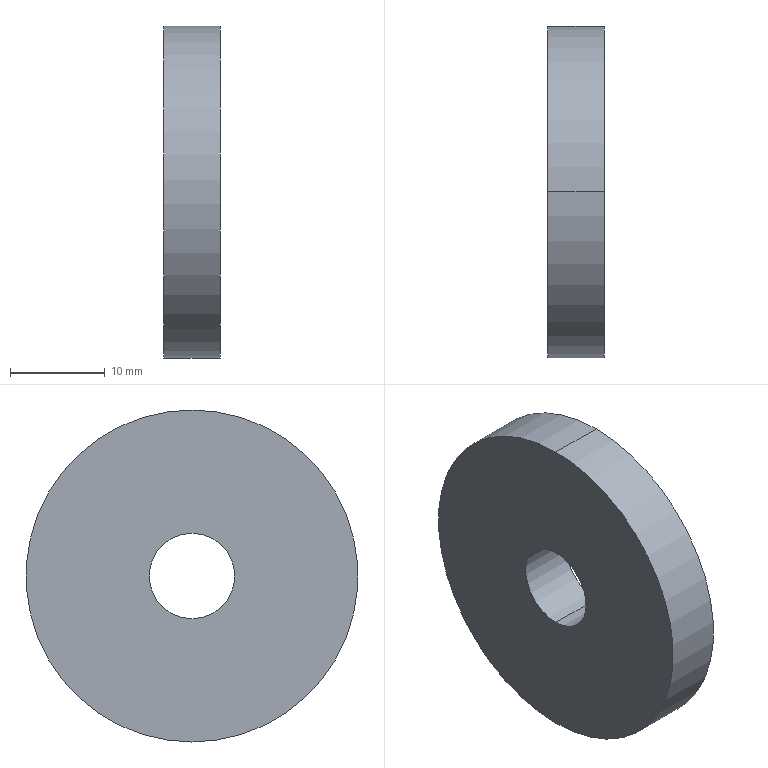Part | SolidWorks | features Extrusion 1 | 1 solid | 6 faces | box 6 x 35 x 35 mm | volume 5391 mm3 | cylinder 4 | plane 2 | commonest cylinder face diameters 9 x2 35 x2
STEP:
#1=CARTESIAN_POINT('',(6.,0.,4.5));
#2=VERTEX_POINT('',#1);
#3=CARTESIAN_POINT('',(6.,0.,-4.5));
#4=VERTEX_POINT('',#3);
#5=CARTESIAN_POINT('',(6.,0.,0.));
#6=DIRECTION('',(1.,0.,0.));
#7=DIRECTION('',(0.,0.,-1.));
#8=AXIS2_PLACEMENT_3D('',#5,#6,#7);
#9=CIRCLE('',#8,4.5);
#10=EDGE_CURVE('',#2,#4,#9,.T.);
#11=ORIENTED_EDGE('',*,*,#10,.T.);
#12=CARTESIAN_POINT('',(0.,0.,-4.5));
#13=VERTEX_POINT('',#12);
#14=CARTESIAN_POINT('',(6.,0.,-4.5));
#15=DIRECTION('',(-1.,0.,0.));
#16=VECTOR('',#15,1000.);
#17=LINE('',#14,#16);
#18=EDGE_CURVE('',#4,#13,#17,.T.);
#19=ORIENTED_EDGE('',*,*,#18,.T.);
#20=CARTESIAN_POINT('',(0.,0.,4.5));
#21=VERTEX_POINT('',#20);
#22=CARTESIAN_POINT('',(0.,0.,0.));
#23=DIRECTION('',(1.,0.,0.));
#24=DIRECTION('',(0.,0.,-1.));
#25=AXIS2_PLACEMENT_3D('',#22,#23,#24);
#26=CIRCLE('',#25,4.5);
#27=EDGE_CURVE('',#21,#13,#26,.T.);
#28=ORIENTED_EDGE('',*,*,#27,.F.);
#29=CARTESIAN_POINT('',(6.,0.,4.5));
#30=DIRECTION('',(-1.,0.,0.));
#31=VECTOR('',#30,1000.);
#32=LINE('',#29,#31);
#33=EDGE_CURVE('',#2,#21,#32,.T.);
#34=ORIENTED_EDGE('',*,*,#33,.F.);
#35=EDGE_LOOP('',(#11,#19,#28,#34));
#36=FACE_OUTER_BOUND('',#35,.T.);
#37=CARTESIAN_POINT('',(6.,0.,0.));
#38=DIRECTION('',(-1.,0.,0.));
#39=DIRECTION('',(0.,0.,1.));
#40=AXIS2_PLACEMENT_3D('',#37,#38,#39);
#41=CYLINDRICAL_SURFACE('',#40,4.5);
#42=ADVANCED_FACE('',(#36),#41,.F.);
#43=CARTESIAN_POINT('',(6.,0.,-17.5));
#44=VERTEX_POINT('',#43);
#45=CARTESIAN_POINT('',(6.,0.,17.5));
#46=VERTEX_POINT('',#45);
#47=CARTESIAN_POINT('',(6.,0.,0.));
#48=DIRECTION('',(1.,0.,0.));
#49=DIRECTION('',(0.,0.,-1.));
#50=AXIS2_PLACEMENT_3D('',#47,#48,#49);
#51=CIRCLE('',#50,17.5);
#52=EDGE_CURVE('',#44,#46,#51,.T.);
#53=ORIENTED_EDGE('',*,*,#52,.F.);
#54=CARTESIAN_POINT('',(0.,0.,-17.5));
#55=VERTEX_POINT('',#54);
#56=CARTESIAN_POINT('',(6.,0.,-17.5));
#57=DIRECTION('',(-1.,0.,0.));
#58=VECTOR('',#57,1000.);
#59=LINE('',#56,#58);
#60=EDGE_CURVE('',#44,#55,#59,.T.);
#61=ORIENTED_EDGE('',*,*,#60,.T.);
#62=CARTESIAN_POINT('',(0.,0.,17.5));
#63=VERTEX_POINT('',#62);
#64=CARTESIAN_POINT('',(0.,0.,0.));
#65=DIRECTION('',(1.,0.,0.));
#66=DIRECTION('',(0.,0.,-1.));
#67=AXIS2_PLACEMENT_3D('',#64,#65,#66);
#68=CIRCLE('',#67,17.5);
#69=EDGE_CURVE('',#55,#63,#68,.T.);
#70=ORIENTED_EDGE('',*,*,#69,.T.);
#71=CARTESIAN_POINT('',(6.,0.,17.5));
#72=DIRECTION('',(-1.,0.,0.));
#73=VECTOR('',#72,1000.);
#74=LINE('',#71,#73);
#75=EDGE_CURVE('',#46,#63,#74,.T.);
#76=ORIENTED_EDGE('',*,*,#75,.F.);
#77=EDGE_LOOP('',(#53,#61,#70,#76));
#78=FACE_OUTER_BOUND('',#77,.T.);
#79=CARTESIAN_POINT('',(6.,0.,0.));
#80=DIRECTION('',(-1.,0.,0.));
#81=DIRECTION('',(0.,0.,1.));
#82=AXIS2_PLACEMENT_3D('',#79,#80,#81);
#83=CYLINDRICAL_SURFACE('',#82,17.5);
#84=ADVANCED_FACE('',(#78),#83,.T.);
#85=CARTESIAN_POINT('',(6.,0.,0.));
#86=DIRECTION('',(1.,0.,0.));
#87=DIRECTION('',(0.,0.,-1.));
#88=AXIS2_PLACEMENT_3D('',#85,#86,#87);
#89=CIRCLE('',#88,17.5);
#90=EDGE_CURVE('',#46,#44,#89,.T.);
#91=ORIENTED_EDGE('',*,*,#90,.T.);
#92=ORIENTED_EDGE('',*,*,#52,.T.);
#93=EDGE_LOOP('',(#91,#92));
#94=FACE_OUTER_BOUND('',#93,.T.);
#95=ORIENTED_EDGE('',*,*,#10,.F.);
#96=CARTESIAN_POINT('',(6.,0.,0.));
#97=DIRECTION('',(1.,0.,0.));
#98=DIRECTION('',(0.,0.,-1.));
#99=AXIS2_PLACEMENT_3D('',#96,#97,#98);
#100=CIRCLE('',#99,4.5);
#101=EDGE_CURVE('',#4,#2,#100,.T.);
#102=ORIENTED_EDGE('',*,*,#101,.F.);
#103=EDGE_LOOP('',(#95,#102));
#104=FACE_BOUND('',#103,.T.);
#105=CARTESIAN_POINT('',(6.,0.,0.));
#106=DIRECTION('',(1.,0.,0.));
#107=DIRECTION('',(0.,0.,-1.));
#108=AXIS2_PLACEMENT_3D('',#105,#106,#107);
#109=PLANE('',#108);
#110=ADVANCED_FACE('',(#94,#104),#109,.T.);
#111=CARTESIAN_POINT('',(0.,0.,0.));
#112=DIRECTION('',(1.,0.,0.));
#113=DIRECTION('',(0.,0.,-1.));
#114=AXIS2_PLACEMENT_3D('',#111,#112,#113);
#115=CIRCLE('',#114,17.5);
#116=EDGE_CURVE('',#63,#55,#115,.T.);
#117=ORIENTED_EDGE('',*,*,#116,.F.);
#118=ORIENTED_EDGE('',*,*,#69,.F.);
#119=EDGE_LOOP('',(#117,#118));
#120=FACE_OUTER_BOUND('',#119,.T.);
#121=ORIENTED_EDGE('',*,*,#27,.T.);
#122=CARTESIAN_POINT('',(0.,0.,0.));
#123=DIRECTION('',(1.,0.,0.));
#124=DIRECTION('',(0.,0.,-1.));
#125=AXIS2_PLACEMENT_3D('',#122,#123,#124);
#126=CIRCLE('',#125,4.5);
#127=EDGE_CURVE('',#13,#21,#126,.T.);
#128=ORIENTED_EDGE('',*,*,#127,.T.);
#129=EDGE_LOOP('',(#121,#128));
#130=FACE_BOUND('',#129,.T.);
#131=CARTESIAN_POINT('',(0.,0.,0.));
#132=DIRECTION('',(1.,0.,0.));
#133=DIRECTION('',(0.,0.,-1.));
#134=AXIS2_PLACEMENT_3D('',#131,#132,#133);
#135=PLANE('',#134);
#136=ADVANCED_FACE('',(#120,#130),#135,.F.);
#137=ORIENTED_EDGE('',*,*,#60,.F.);
#138=ORIENTED_EDGE('',*,*,#90,.F.);
#139=ORIENTED_EDGE('',*,*,#75,.T.);
#140=ORIENTED_EDGE('',*,*,#116,.T.);
#141=EDGE_LOOP('',(#137,#138,#139,#140));
#142=FACE_OUTER_BOUND('',#141,.T.);
#143=CARTESIAN_POINT('',(6.,0.,0.));
#144=DIRECTION('',(-1.,0.,0.));
#145=DIRECTION('',(0.,0.,1.));
#146=AXIS2_PLACEMENT_3D('',#143,#144,#145);
#147=CYLINDRICAL_SURFACE('',#146,17.5);
#148=ADVANCED_FACE('',(#142),#147,.T.);
#149=ORIENTED_EDGE('',*,*,#18,.F.);
#150=ORIENTED_EDGE('',*,*,#101,.T.);
#151=ORIENTED_EDGE('',*,*,#33,.T.);
#152=ORIENTED_EDGE('',*,*,#127,.F.);
#153=EDGE_LOOP('',(#149,#150,#151,#152));
#154=FACE_OUTER_BOUND('',#153,.T.);
#155=CARTESIAN_POINT('',(6.,0.,0.));
#156=DIRECTION('',(-1.,0.,0.));
#157=DIRECTION('',(0.,0.,1.));
#158=AXIS2_PLACEMENT_3D('',#155,#156,#157);
#159=CYLINDRICAL_SURFACE('',#158,4.5);
#160=ADVANCED_FACE('',(#154),#159,.F.);
#161=CLOSED_SHELL('',(#42,#84,#110,#136,#148,#160));
#162=MANIFOLD_SOLID_BREP('',#161);
#163=CARTESIAN_POINT('',(0.,0.,0.));
#164=DIRECTION('',(0.,0.,1.));
#165=DIRECTION('',(1.,0.,0.));
#166=AXIS2_PLACEMENT_3D('',#163,#164,#165);
#167=(LENGTH_UNIT()NAMED_UNIT(*)SI_UNIT(.MILLI.,.METRE.));
#168=UNCERTAINTY_MEASURE_WITH_UNIT(LENGTH_MEASURE(0.00001),#167,'','');
#169=(NAMED_UNIT(*)PLANE_ANGLE_UNIT()SI_UNIT($,.RADIAN.));
#170=(NAMED_UNIT(*)SI_UNIT($,.STERADIAN.)SOLID_ANGLE_UNIT());
#171=(GEOMETRIC_REPRESENTATION_CONTEXT(3)GLOBAL_UNCERTAINTY_ASSIGNED_CONTEXT((#168))GLOBAL_UNIT_ASSIGNED_CONTEXT((#167,#169,#170))REPRESENTATION_CONTEXT('',''));
#172=ADVANCED_BREP_SHAPE_REPRESENTATION('',(#162,#166),#171);